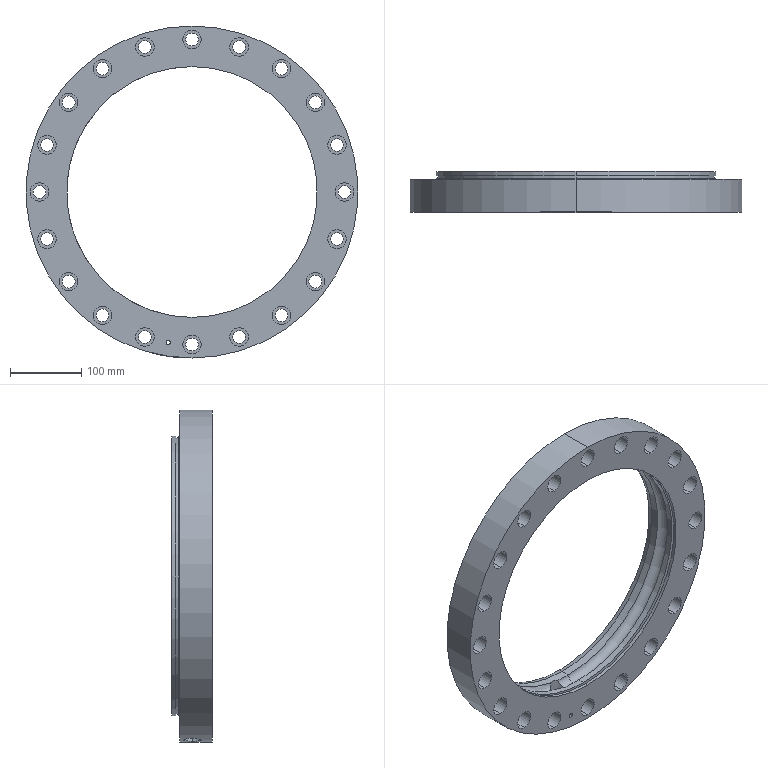Part | SolidWorks | features ICE 2, CirPattern 1, HoleWzd 1, RefAxis 1, Revolution 1 | 1 solid | 140 faces | box 466 x 57 x 466 mm | volume 2930059 mm3 | cylinder 106 | plane 29 | torus 3 | cone 2 | commonest cylinder face diameters 18 x40 26 x40 6 x4 352 x4 392 x4 25 x2